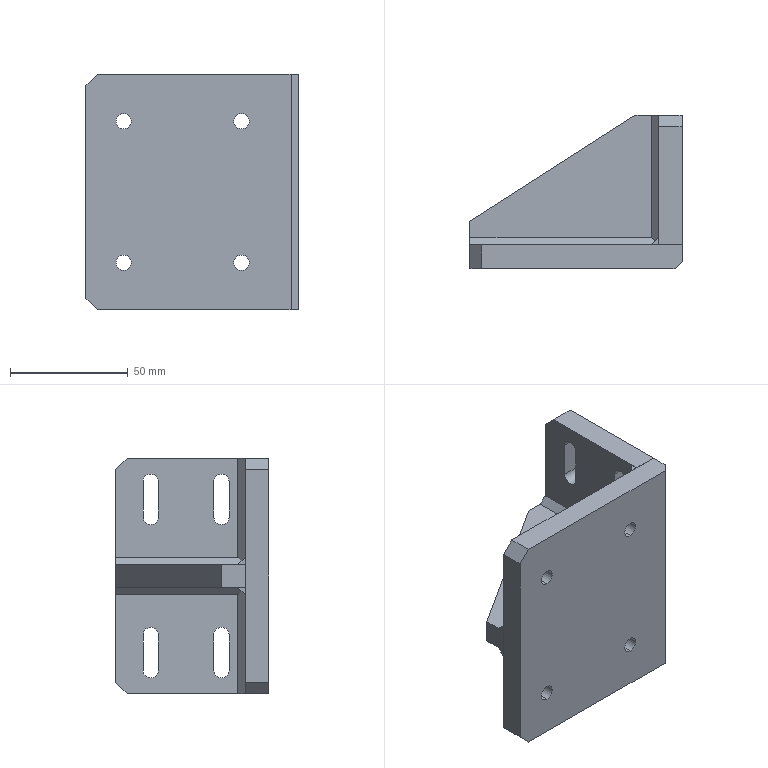Part | STEP file | 866-BDO024-91-11A_default_machined_ | 6 solids | 71 faces | box 90 x 65 x 100 mm | volume 167392 mm3 | plane 51 | cylinder 20 | commonest cylinder face diameters 6.5 x20